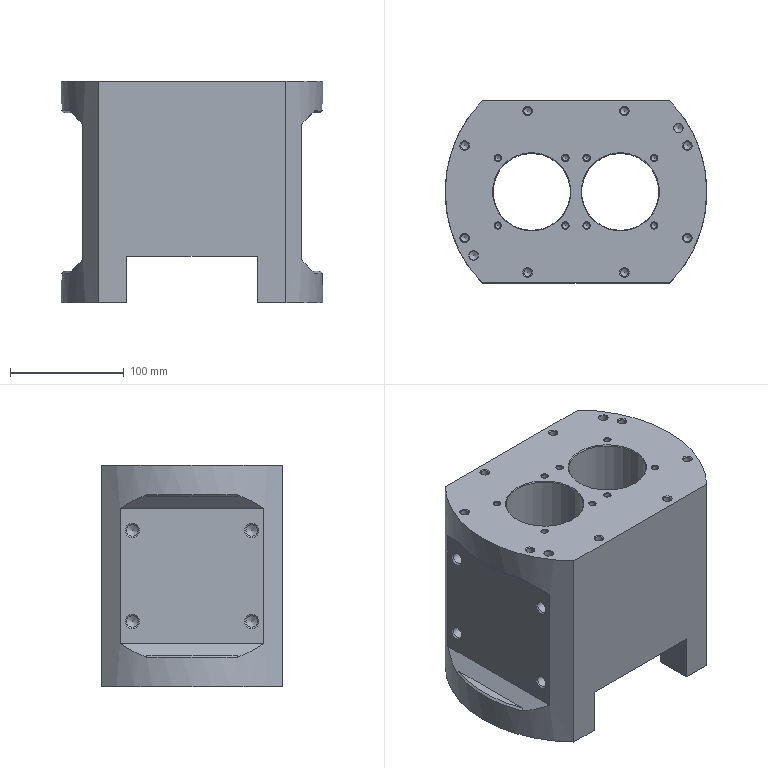NC program | NX | posted with a generic post | part box 230 x 160 x 195 mm
Lines 1 to 132 of 1674:
N10 G17 G21 G94 G90
(FLOOR_WALL_COPY_COPY_COPY_COPY_1 , TOOL : D50)
N12 T02 M6
N14 G54
N16 G17 G0 G90 X-118.531 Y79.997 B0. C0. S2500 M3
N18 G43 Z30. H2
N20 Z3.
N22 G94 G1 Z0. F1000.
N24 X-114.893
N26 X114.893
N28 G2 X132.571 Y44.998 R140.
N30 G1 X-132.571
N32 G3 X-139.643 Y9.999 R140.
N34 G1 X139.643
N36 G2 X137.75 Y-25.001 R140.
N38 G1 X-137.75
N40 G3 X-136.717 Y-30.141 R140.
N42 X-136.567 Y-30.811 R138.505
N44 X-136.489 Y-31.156 R139.262
N46 X-136.433 Y-31.4 R138.778
N48 X-126.491 Y-60. R140.
N50 G1 X126.491
N52 X129.804
N54 Z3.
N56 G0 Z30.
N58 M5
(DRILLING_COPY_2 , TOOL : ZXZ)
N60 T01 M6
N62 G54
N64 G17 G0 G90 X-42.5 Y-71. B0. C0. S5000 M3
N66 G43 Z30. H1
N68 G94 G81 G98 Z-1. F250. R3.
N70 X-90. Y-56.
N72 X-97.931 Y-40.564
N74 X-68.698 Y-29.698
N76 X-39. Y0.
N78 X-9.302 Y-29.698
N80 X9.302
N82 X42.5 Y-71.
N84 X97.931 Y-40.564
N86 X68.698 Y-29.698
N88 X39. Y0.
N90 X68.698 Y29.698
N92 X97.931 Y40.564
N94 X90. Y56.
N96 X42.5 Y71.
N98 X9.302 Y29.698
N100 X-9.302
N102 X-42.5 Y71.
N104 X-68.698 Y29.698
N106 X-97.931 Y40.564
N108 G80
N110 G0 X-97.931 Y40.564 Z30.
N112 M5
(DRILLING_COPY_2_COPY , TOOL : 6.8ZT)
N114 T16 M6
N116 G54
N118 G17 G0 G90 X-42.5 Y-71. B0. C0. S2000 M3
N120 G43 Z30. H16
N122 G94 G83 G98 Z-27.043 F200. Q2. R3.
N124 X-97.931 Y-40.564
N126 Y40.564
N128 X-42.5 Y71.
N130 X42.5
N132 X97.931 Y40.564
N134 Y-40.564
N136 X42.5 Y-71.
N138 G80
N140 G0 X42.5 Y-71. Z30.
N142 M5
(DRILLING_COPY_2_COPY_COPY_1 , TOOL : 5.2ZT)
N144 T15 M6
N146 G54
N148 G17 G0 G90 X9.302 Y29.698 B0. C0. S2000 M3
N150 G43 Z30. H15
N152 G94 G83 G98 Z-21.502 F200. Q2. R3.
N154 X-9.302
N156 X-68.698
N158 Y-29.698
N160 X-9.302
N162 X9.302
N164 X68.698
N166 Y29.698
N168 G80
N170 G0 X68.698 Y29.698 Z30.
N172 M5
(DRILLING_COPY_2_COPY_COPY_1_COPY_1 , TOOL : 7.8ZT)
N174 T17 M6
N176 G54
N178 G17 G0 G90 X90. Y56. B0. C0. S2000 M3
N180 G43 Z30. H17
N182 G94 G83 G98 Z-22.403 F200. Q2. R3.
N184 X-90. Y-56.
N186 G80
N188 G0 X-90. Y-56. Z30.
N190 M5
(DRILLING_COPY_2_COPY_COPY_1_COPY_1_COPY , TOOL : 8.0JD)
N192 T18 M6
N194 G54
N196 G17 G0 G90 X90. Y56. B0. C0. S1000 M3
N198 G43 Z30. H18
N200 G94 G85 G98 Z-20. F40. R3.
N202 X-90. Y-56.
N204 G80
N206 G0 X-90. Y-56. Z30.
N208 M5
(DRILLING_COPY_COPY_1_COPY , TOOL : 11.8ZT)
N210 T19 M6
N212 G54
N214 G17 G0 G90 X-39. Y0. B0. C0. S1025 M3
N216 G43 Z30. H19
N218 G94 G83 G98 Z-159.045 F150. Q2. R2.
N220 X39. R3.
N222 G80
N224 G0 X39. Y0. Z30.
N226 M5